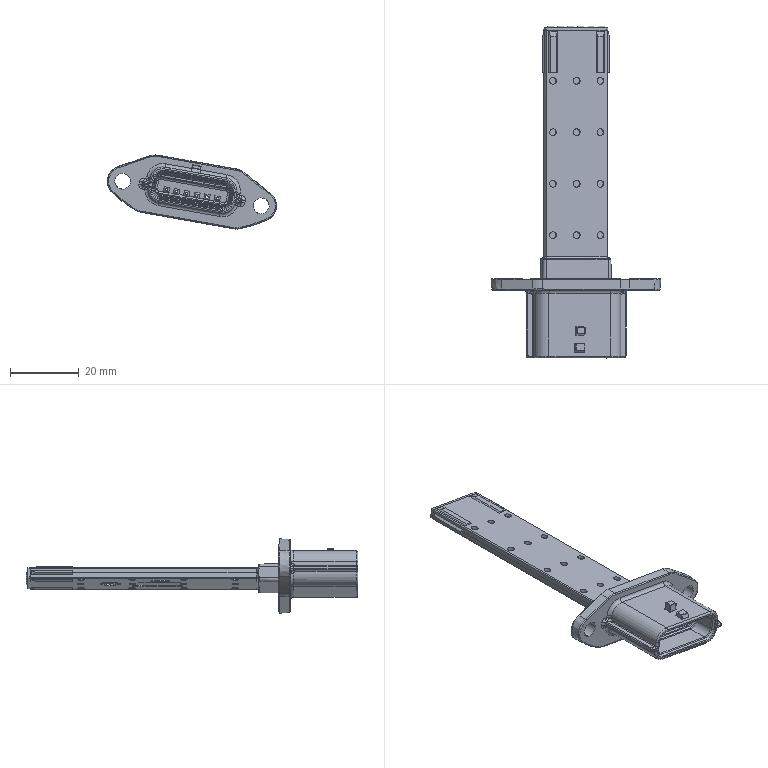Part | SolidWorks | features BaseBody 1 | 1 solid | 1384 faces | box 49.369 x 96.8 x 21.617 mm | volume 9085 mm3 | plane 974 | cylinder 262 | torus 73 | spline 39 | cone 18 | sphere 18 | commonest cylinder face diameters 2 x90 0.2 x83 0.6 x22 1 x16 0.5 x10 0.3 x8